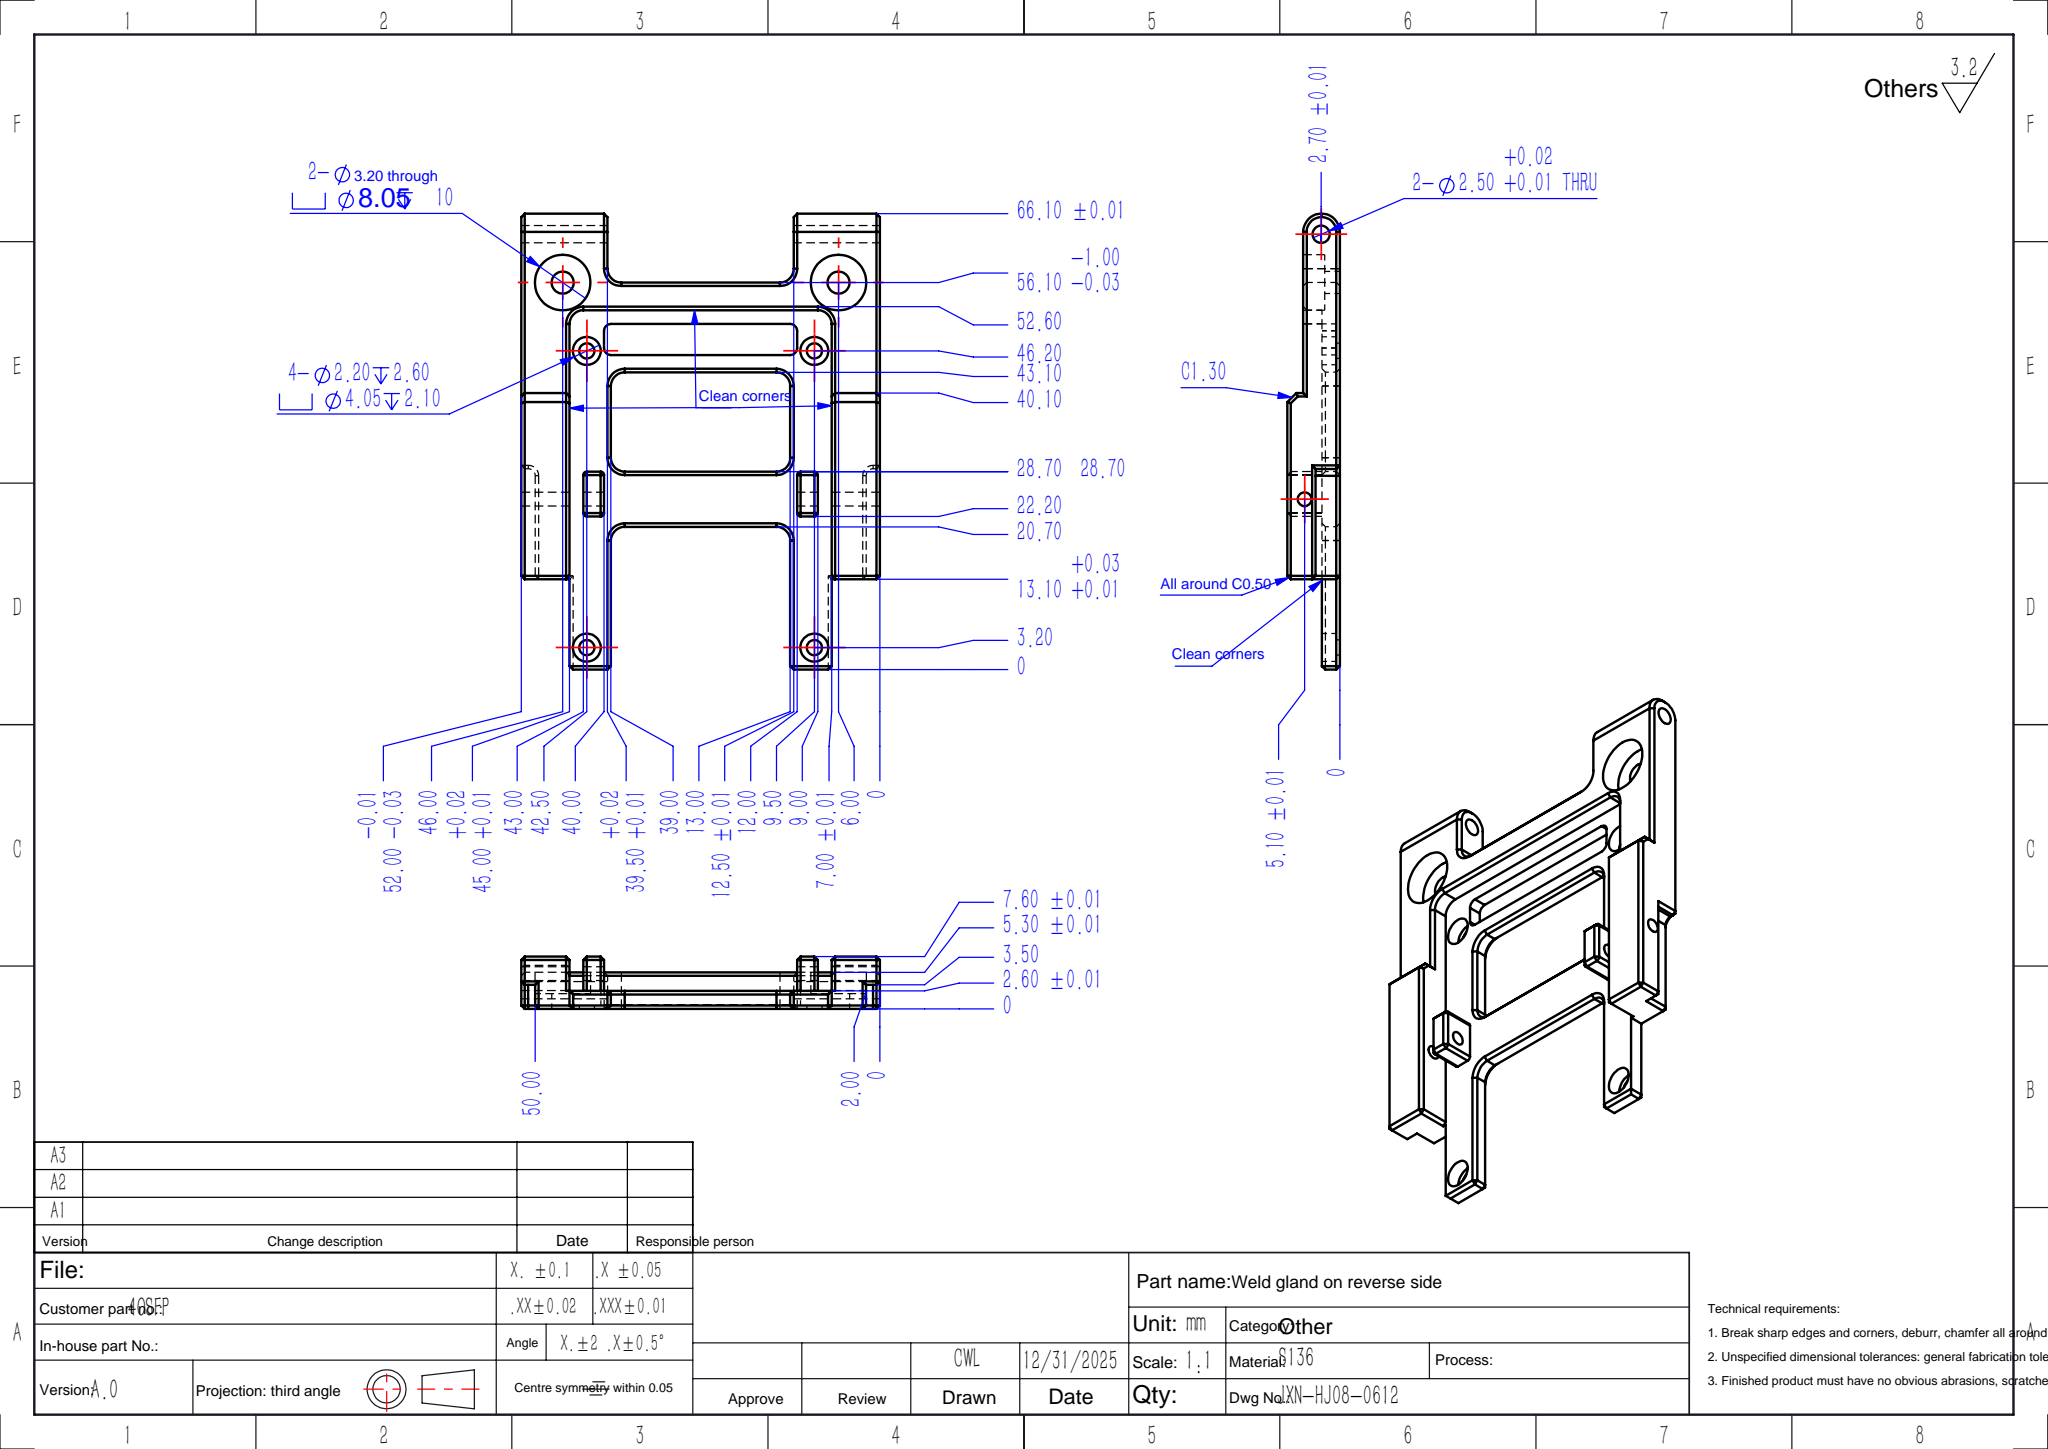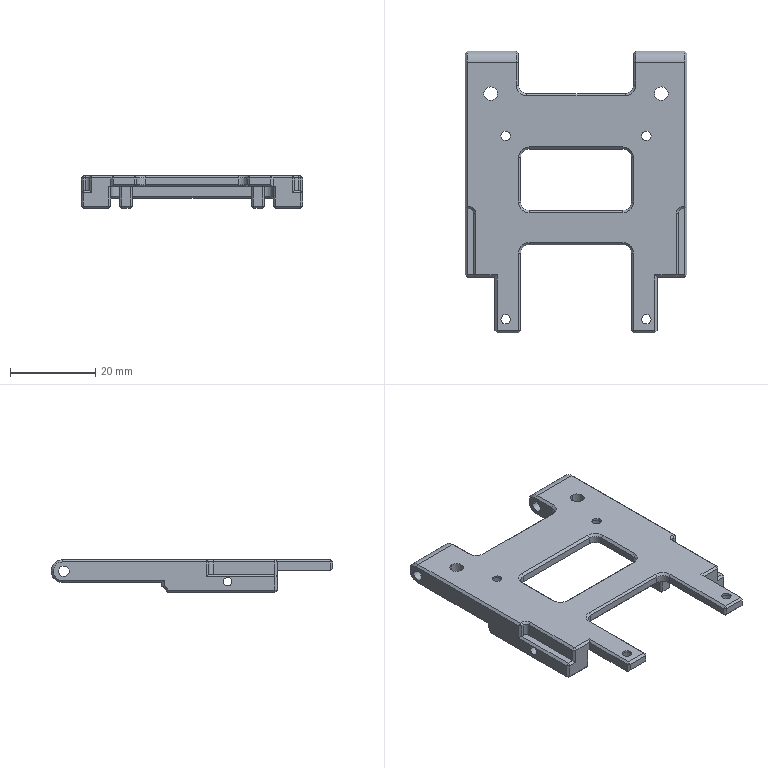Part | SolidWorks | features ICE 17, Fillet 6, Chamfer 2, MoveFace 2, Extrusion 1 | 1 solid | 250 faces | box 52 x 66.1 x 7.6 mm | volume 7860 mm3 | plane 150 | cylinder 64 | cone 36 | commonest cylinder face diameters 2 x14 4 x10 1 x8 2.2 x8 4.05 x8 2.5 x4